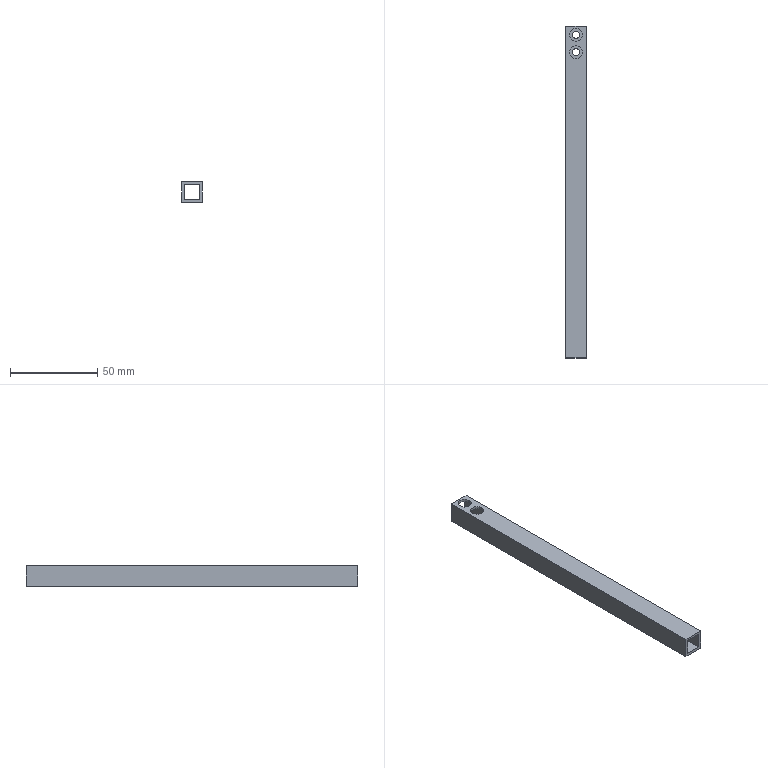Part | STEP file | B1-010 | 1 solid | 18 faces | box 12 x 190 x 12 mm | volume 11800 mm3 | plane 10 | cylinder 8 | commonest cylinder face diameters 4 x4 7.5 x4
STEP:
#1=CARTESIAN_POINT('',(0.,0.,0.));
#2=DIRECTION('',(0.,0.,1.));
#3=DIRECTION('',(1.,0.,0.));
#4=AXIS2_PLACEMENT_3D('',#1,#2,#3);
#5=CARTESIAN_POINT('',(3.75,80.,4.5));
#6=VERTEX_POINT('',#5);
#7=CARTESIAN_POINT('',(3.75,80.,6.));
#8=VERTEX_POINT('',#7);
#9=CARTESIAN_POINT('',(3.75,80.,-6.001));
#10=DIRECTION('',(0.,0.,1.));
#11=VECTOR('',#10,1.);
#12=LINE('',#9,#11);
#13=CARTESIAN_POINT('',(0.,80.,-6.001));
#14=DIRECTION('',(0.,0.,1.));
#15=DIRECTION('',(1.,0.,0.));
#16=AXIS2_PLACEMENT_3D('',#13,#14,#15);
#17=CYLINDRICAL_SURFACE('',#16,3.75);
#18=CARTESIAN_POINT('',(6.283,0.));
#19=DIRECTION('',(0.,1.));
#20=VECTOR('',#19,1.);
#21=LINE('',#18,#20);
#22=(GEOMETRIC_REPRESENTATION_CONTEXT(2)PARAMETRIC_REPRESENTATION_CONTEXT()REPRESENTATION_CONTEXT('',''));
#23=DEFINITIONAL_REPRESENTATION('',(#21),#22);
#24=PCURVE('',#17,#23);
#25=CARTESIAN_POINT('',(0.,80.,-6.001));
#26=DIRECTION('',(0.,0.,1.));
#27=DIRECTION('',(1.,0.,0.));
#28=AXIS2_PLACEMENT_3D('',#25,#26,#27);
#29=CYLINDRICAL_SURFACE('',#28,3.75);
#30=CARTESIAN_POINT('',(0.,0.));
#31=DIRECTION('',(0.,1.));
#32=VECTOR('',#31,1.);
#33=LINE('',#30,#32);
#34=(GEOMETRIC_REPRESENTATION_CONTEXT(2)PARAMETRIC_REPRESENTATION_CONTEXT()REPRESENTATION_CONTEXT('',''));
#35=DEFINITIONAL_REPRESENTATION('',(#33),#34);
#36=PCURVE('',#29,#35);
#37=SURFACE_CURVE('',#12,(#24,#36),.PCURVE_S1.);
#38=EDGE_CURVE('',#6,#8,#37,.T.);
#39=ORIENTED_EDGE('',*,*,#38,.T.);
#40=CARTESIAN_POINT('',(-3.75,80.,6.));
#41=VERTEX_POINT('',#40);
#42=CARTESIAN_POINT('',(0.,80.,6.));
#43=DIRECTION('',(0.,0.,1.));
#44=DIRECTION('',(1.,0.,0.));
#45=AXIS2_PLACEMENT_3D('',#42,#43,#44);
#46=CIRCLE('',#45,3.75);
#47=CARTESIAN_POINT('',(0.,12.001));
#48=DIRECTION('',(1.,0.));
#49=VECTOR('',#48,1.);
#50=LINE('',#47,#49);
#51=(GEOMETRIC_REPRESENTATION_CONTEXT(2)PARAMETRIC_REPRESENTATION_CONTEXT()REPRESENTATION_CONTEXT('',''));
#52=DEFINITIONAL_REPRESENTATION('',(#50),#51);
#53=PCURVE('',#17,#52);
#54=CARTESIAN_POINT('',(-6.,95.,6.));
#55=DIRECTION('',(0.,0.,-1.));
#56=DIRECTION('',(-1.,0.,0.));
#57=AXIS2_PLACEMENT_3D('',#54,#55,#56);
#58=PLANE('',#57);
#59=CARTESIAN_POINT('',(-9.75,-15.));
#60=CARTESIAN_POINT('',(-9.75,-8.505));
#61=CARTESIAN_POINT('',(-4.125,-11.752));
#62=CARTESIAN_POINT('',(1.5,-15.));
#63=CARTESIAN_POINT('',(-4.125,-18.248));
#64=CARTESIAN_POINT('',(-9.75,-21.495));
#65=CARTESIAN_POINT('',(-9.75,-15.));
#66=(BOUNDED_CURVE()B_SPLINE_CURVE(2,(#59,#60,#61,#62,#63,#64,#65),.UNSPECIFIED.,.T.,.F.)B_SPLINE_CURVE_WITH_KNOTS((1,2,2,2,2,1),(-2.094,0.,2.094,4.189,6.283,8.378),.UNSPECIFIED.)CURVE()GEOMETRIC_REPRESENTATION_ITEM()RATIONAL_B_SPLINE_CURVE((1.,0.5,1.,0.5,1.,0.5,1.))REPRESENTATION_ITEM(''));
#67=(GEOMETRIC_REPRESENTATION_CONTEXT(2)PARAMETRIC_REPRESENTATION_CONTEXT()REPRESENTATION_CONTEXT('',''));
#68=DEFINITIONAL_REPRESENTATION('',(#66),#67);
#69=PCURVE('',#58,#68);
#70=SURFACE_CURVE('',#46,(#53,#69),.PCURVE_S1.);
#71=EDGE_CURVE('',#41,#8,#70,.T.);
#72=ORIENTED_EDGE('',*,*,#71,.F.);
#73=CARTESIAN_POINT('',(-3.75,80.,4.5));
#74=VERTEX_POINT('',#73);
#75=CARTESIAN_POINT('',(-3.75,80.,-6.001));
#76=DIRECTION('',(0.,0.,1.));
#77=VECTOR('',#76,1.);
#78=LINE('',#75,#77);
#79=CARTESIAN_POINT('',(3.142,0.));
#80=DIRECTION('',(0.,1.));
#81=VECTOR('',#80,1.);
#82=LINE('',#79,#81);
#83=(GEOMETRIC_REPRESENTATION_CONTEXT(2)PARAMETRIC_REPRESENTATION_CONTEXT()REPRESENTATION_CONTEXT('',''));
#84=DEFINITIONAL_REPRESENTATION('',(#82),#83);
#85=PCURVE('',#17,#84);
#86=CARTESIAN_POINT('',(3.142,0.));
#87=DIRECTION('',(0.,1.));
#88=VECTOR('',#87,1.);
#89=LINE('',#86,#88);
#90=(GEOMETRIC_REPRESENTATION_CONTEXT(2)PARAMETRIC_REPRESENTATION_CONTEXT()REPRESENTATION_CONTEXT('',''));
#91=DEFINITIONAL_REPRESENTATION('',(#89),#90);
#92=PCURVE('',#29,#91);
#93=SURFACE_CURVE('',#78,(#85,#92),.PCURVE_S1.);
#94=EDGE_CURVE('',#74,#41,#93,.T.);
#95=ORIENTED_EDGE('',*,*,#94,.F.);
#96=CARTESIAN_POINT('',(0.,80.,4.5));
#97=DIRECTION('',(0.,0.,1.));
#98=DIRECTION('',(-1.,0.,0.));
#99=AXIS2_PLACEMENT_3D('',#96,#97,#98);
#100=CIRCLE('',#99,3.75);
#101=CARTESIAN_POINT('',(3.142,10.501));
#102=DIRECTION('',(1.,0.));
#103=VECTOR('',#102,1.);
#104=LINE('',#101,#103);
#105=(GEOMETRIC_REPRESENTATION_CONTEXT(2)PARAMETRIC_REPRESENTATION_CONTEXT()REPRESENTATION_CONTEXT('',''));
#106=DEFINITIONAL_REPRESENTATION('',(#104),#105);
#107=PCURVE('',#17,#106);
#108=CARTESIAN_POINT('',(-4.5,95.,4.5));
#109=DIRECTION('',(0.,0.,-1.));
#110=DIRECTION('',(-1.,0.,0.));
#111=AXIS2_PLACEMENT_3D('',#108,#109,#110);
#112=PLANE('',#111);
#113=CARTESIAN_POINT('',(-0.75,-15.));
#114=CARTESIAN_POINT('',(-0.75,-21.495));
#115=CARTESIAN_POINT('',(-6.375,-18.248));
#116=CARTESIAN_POINT('',(-12.,-15.));
#117=CARTESIAN_POINT('',(-6.375,-11.752));
#118=CARTESIAN_POINT('',(-0.75,-8.505));
#119=CARTESIAN_POINT('',(-0.75,-15.));
#120=(BOUNDED_CURVE()B_SPLINE_CURVE(2,(#113,#114,#115,#116,#117,#118,#119),.UNSPECIFIED.,.T.,.F.)B_SPLINE_CURVE_WITH_KNOTS((1,2,2,2,2,1),(-2.094,0.,2.094,4.189,6.283,8.378),.UNSPECIFIED.)CURVE()GEOMETRIC_REPRESENTATION_ITEM()RATIONAL_B_SPLINE_CURVE((1.,0.5,1.,0.5,1.,0.5,1.))REPRESENTATION_ITEM(''));
#121=(GEOMETRIC_REPRESENTATION_CONTEXT(2)PARAMETRIC_REPRESENTATION_CONTEXT()REPRESENTATION_CONTEXT('',''));
#122=DEFINITIONAL_REPRESENTATION('',(#120),#121);
#123=PCURVE('',#112,#122);
#124=SURFACE_CURVE('',#100,(#107,#123),.PCURVE_S1.);
#125=EDGE_CURVE('',#74,#6,#124,.T.);
#126=ORIENTED_EDGE('',*,*,#125,.T.);
#127=EDGE_LOOP('',(#39,#72,#95,#126));
#128=FACE_BOUND('',#127,.F.);
#129=ADVANCED_FACE('',(#128),#17,.F.);
#130=CARTESIAN_POINT('',(2.,80.,-6.));
#131=VERTEX_POINT('',#130);
#132=CARTESIAN_POINT('',(2.,80.,-4.5));
#133=VERTEX_POINT('',#132);
#134=CARTESIAN_POINT('',(2.,80.,-6.));
#135=DIRECTION('',(0.,0.,1.));
#136=VECTOR('',#135,1.);
#137=LINE('',#134,#136);
#138=CARTESIAN_POINT('',(0.,80.,-6.));
#139=DIRECTION('',(0.,0.,1.));
#140=DIRECTION('',(1.,0.,0.));
#141=AXIS2_PLACEMENT_3D('',#138,#139,#140);
#142=CYLINDRICAL_SURFACE('',#141,2.);
#143=CARTESIAN_POINT('',(6.283,0.));
#144=DIRECTION('',(0.,1.));
#145=VECTOR('',#144,1.);
#146=LINE('',#143,#145);
#147=(GEOMETRIC_REPRESENTATION_CONTEXT(2)PARAMETRIC_REPRESENTATION_CONTEXT()REPRESENTATION_CONTEXT('',''));
#148=DEFINITIONAL_REPRESENTATION('',(#146),#147);
#149=PCURVE('',#142,#148);
#150=CARTESIAN_POINT('',(0.,80.,-6.));
#151=DIRECTION('',(0.,0.,1.));
#152=DIRECTION('',(1.,0.,0.));
#153=AXIS2_PLACEMENT_3D('',#150,#151,#152);
#154=CYLINDRICAL_SURFACE('',#153,2.);
#155=CARTESIAN_POINT('',(0.,0.));
#156=DIRECTION('',(0.,1.));
#157=VECTOR('',#156,1.);
#158=LINE('',#155,#157);
#159=(GEOMETRIC_REPRESENTATION_CONTEXT(2)PARAMETRIC_REPRESENTATION_CONTEXT()REPRESENTATION_CONTEXT('',''));
#160=DEFINITIONAL_REPRESENTATION('',(#158),#159);
#161=PCURVE('',#154,#160);
#162=SURFACE_CURVE('',#137,(#149,#161),.PCURVE_S1.);
#163=EDGE_CURVE('',#131,#133,#162,.T.);
#164=ORIENTED_EDGE('',*,*,#163,.T.);
#165=CARTESIAN_POINT('',(-2.,80.,-4.5));
#166=VERTEX_POINT('',#165);
#167=CARTESIAN_POINT('',(0.,80.,-4.5));
#168=DIRECTION('',(0.,0.,1.));
#169=DIRECTION('',(1.,0.,0.));
#170=AXIS2_PLACEMENT_3D('',#167,#168,#169);
#171=CIRCLE('',#170,2.);
#172=CARTESIAN_POINT('',(0.,1.5));
#173=DIRECTION('',(1.,0.));
#174=VECTOR('',#173,1.);
#175=LINE('',#172,#174);
#176=(GEOMETRIC_REPRESENTATION_CONTEXT(2)PARAMETRIC_REPRESENTATION_CONTEXT()REPRESENTATION_CONTEXT('',''));
#177=DEFINITIONAL_REPRESENTATION('',(#175),#176);
#178=PCURVE('',#142,#177);
#179=CARTESIAN_POINT('',(-4.5,95.,-4.5));
#180=DIRECTION('',(0.,0.,1.));
#181=DIRECTION('',(1.,0.,0.));
#182=AXIS2_PLACEMENT_3D('',#179,#180,#181);
#183=PLANE('',#182);
#184=CARTESIAN_POINT('',(4.5,-15.));
#185=DIRECTION('',(1.,0.));
#186=AXIS2_PLACEMENT_2D('',#184,#185);
#187=CIRCLE('',#186,2.);
#188=(GEOMETRIC_REPRESENTATION_CONTEXT(2)PARAMETRIC_REPRESENTATION_CONTEXT()REPRESENTATION_CONTEXT('',''));
#189=DEFINITIONAL_REPRESENTATION('',(#187),#188);
#190=PCURVE('',#183,#189);
#191=SURFACE_CURVE('',#171,(#178,#190),.PCURVE_S1.);
#192=EDGE_CURVE('',#166,#133,#191,.T.);
#193=ORIENTED_EDGE('',*,*,#192,.F.);
#194=CARTESIAN_POINT('',(-2.,80.,-6.));
#195=VERTEX_POINT('',#194);
#196=CARTESIAN_POINT('',(-2.,80.,-6.));
#197=DIRECTION('',(0.,0.,1.));
#198=VECTOR('',#197,1.);
#199=LINE('',#196,#198);
#200=CARTESIAN_POINT('',(3.142,0.));
#201=DIRECTION('',(0.,1.));
#202=VECTOR('',#201,1.);
#203=LINE('',#200,#202);
#204=(GEOMETRIC_REPRESENTATION_CONTEXT(2)PARAMETRIC_REPRESENTATION_CONTEXT()REPRESENTATION_CONTEXT('',''));
#205=DEFINITIONAL_REPRESENTATION('',(#203),#204);
#206=PCURVE('',#142,#205);
#207=CARTESIAN_POINT('',(3.142,0.));
#208=DIRECTION('',(0.,1.));
#209=VECTOR('',#208,1.);
#210=LINE('',#207,#209);
#211=(GEOMETRIC_REPRESENTATION_CONTEXT(2)PARAMETRIC_REPRESENTATION_CONTEXT()REPRESENTATION_CONTEXT('',''));
#212=DEFINITIONAL_REPRESENTATION('',(#210),#211);
#213=PCURVE('',#154,#212);
#214=SURFACE_CURVE('',#199,(#206,#213),.PCURVE_S1.);
#215=EDGE_CURVE('',#195,#166,#214,.T.);
#216=ORIENTED_EDGE('',*,*,#215,.F.);
#217=CARTESIAN_POINT('',(0.,80.,-6.));
#218=DIRECTION('',(0.,0.,1.));
#219=DIRECTION('',(1.,0.,0.));
#220=AXIS2_PLACEMENT_3D('',#217,#218,#219);
#221=CIRCLE('',#220,2.);
#222=CARTESIAN_POINT('',(0.,0.));
#223=DIRECTION('',(1.,0.));
#224=VECTOR('',#223,1.);
#225=LINE('',#222,#224);
#226=(GEOMETRIC_REPRESENTATION_CONTEXT(2)PARAMETRIC_REPRESENTATION_CONTEXT()REPRESENTATION_CONTEXT('',''));
#227=DEFINITIONAL_REPRESENTATION('',(#225),#226);
#228=PCURVE('',#142,#227);
#229=CARTESIAN_POINT('',(-6.,95.,-6.));
#230=DIRECTION('',(0.,0.,1.));
#231=DIRECTION('',(1.,0.,0.));
#232=AXIS2_PLACEMENT_3D('',#229,#230,#231);
#233=PLANE('',#232);
#234=CARTESIAN_POINT('',(6.,-15.));
#235=DIRECTION('',(1.,0.));
#236=AXIS2_PLACEMENT_2D('',#234,#235);
#237=CIRCLE('',#236,2.);
#238=(GEOMETRIC_REPRESENTATION_CONTEXT(2)PARAMETRIC_REPRESENTATION_CONTEXT()REPRESENTATION_CONTEXT('',''));
#239=DEFINITIONAL_REPRESENTATION('',(#237),#238);
#240=PCURVE('',#233,#239);
#241=SURFACE_CURVE('',#221,(#228,#240),.PCURVE_S1.);
#242=EDGE_CURVE('',#195,#131,#241,.T.);
#243=ORIENTED_EDGE('',*,*,#242,.T.);
#244=EDGE_LOOP('',(#164,#193,#216,#243));
#245=FACE_BOUND('',#244,.F.);
#246=ADVANCED_FACE('',(#245),#142,.F.);
#247=CARTESIAN_POINT('',(3.75,90.,4.5));
#248=VERTEX_POINT('',#247);
#249=CARTESIAN_POINT('',(3.75,90.,6.));
#250=VERTEX_POINT('',#249);
#251=CARTESIAN_POINT('',(3.75,90.,-6.001));
#252=DIRECTION('',(0.,0.,1.));
#253=VECTOR('',#252,1.);
#254=LINE('',#251,#253);
#255=CARTESIAN_POINT('',(0.,90.,-6.001));
#256=DIRECTION('',(0.,0.,1.));
#257=DIRECTION('',(1.,0.,0.));
#258=AXIS2_PLACEMENT_3D('',#255,#256,#257);
#259=CYLINDRICAL_SURFACE('',#258,3.75);
#260=CARTESIAN_POINT('',(6.283,0.));
#261=DIRECTION('',(0.,1.));
#262=VECTOR('',#261,1.);
#263=LINE('',#260,#262);
#264=(GEOMETRIC_REPRESENTATION_CONTEXT(2)PARAMETRIC_REPRESENTATION_CONTEXT()REPRESENTATION_CONTEXT('',''));
#265=DEFINITIONAL_REPRESENTATION('',(#263),#264);
#266=PCURVE('',#259,#265);
#267=CARTESIAN_POINT('',(0.,90.,-6.001));
#268=DIRECTION('',(0.,0.,1.));
#269=DIRECTION('',(1.,0.,0.));
#270=AXIS2_PLACEMENT_3D('',#267,#268,#269);
#271=CYLINDRICAL_SURFACE('',#270,3.75);
#272=CARTESIAN_POINT('',(0.,0.));
#273=DIRECTION('',(0.,1.));
#274=VECTOR('',#273,1.);
#275=LINE('',#272,#274);
#276=(GEOMETRIC_REPRESENTATION_CONTEXT(2)PARAMETRIC_REPRESENTATION_CONTEXT()REPRESENTATION_CONTEXT('',''));
#277=DEFINITIONAL_REPRESENTATION('',(#275),#276);
#278=PCURVE('',#271,#277);
#279=SURFACE_CURVE('',#254,(#266,#278),.PCURVE_S1.);
#280=EDGE_CURVE('',#248,#250,#279,.T.);
#281=ORIENTED_EDGE('',*,*,#280,.T.);
#282=CARTESIAN_POINT('',(-3.75,90.,6.));
#283=VERTEX_POINT('',#282);
#284=CARTESIAN_POINT('',(0.,90.,6.));
#285=DIRECTION('',(0.,0.,1.));
#286=DIRECTION('',(1.,0.,0.));
#287=AXIS2_PLACEMENT_3D('',#284,#285,#286);
#288=CIRCLE('',#287,3.75);
#289=CARTESIAN_POINT('',(0.,12.001));
#290=DIRECTION('',(1.,0.));
#291=VECTOR('',#290,1.);
#292=LINE('',#289,#291);
#293=(GEOMETRIC_REPRESENTATION_CONTEXT(2)PARAMETRIC_REPRESENTATION_CONTEXT()REPRESENTATION_CONTEXT('',''));
#294=DEFINITIONAL_REPRESENTATION('',(#292),#293);
#295=PCURVE('',#259,#294);
#296=CARTESIAN_POINT('',(-9.75,-5.));
#297=CARTESIAN_POINT('',(-9.75,1.495));
#298=CARTESIAN_POINT('',(-4.125,-1.752));
#299=CARTESIAN_POINT('',(1.5,-5.));
#300=CARTESIAN_POINT('',(-4.125,-8.248));
#301=CARTESIAN_POINT('',(-9.75,-11.495));
#302=CARTESIAN_POINT('',(-9.75,-5.));
#303=(BOUNDED_CURVE()B_SPLINE_CURVE(2,(#296,#297,#298,#299,#300,#301,#302),.UNSPECIFIED.,.T.,.F.)B_SPLINE_CURVE_WITH_KNOTS((1,2,2,2,2,1),(-2.094,0.,2.094,4.189,6.283,8.378),.UNSPECIFIED.)CURVE()GEOMETRIC_REPRESENTATION_ITEM()RATIONAL_B_SPLINE_CURVE((1.,0.5,1.,0.5,1.,0.5,1.))REPRESENTATION_ITEM(''));
#304=(GEOMETRIC_REPRESENTATION_CONTEXT(2)PARAMETRIC_REPRESENTATION_CONTEXT()REPRESENTATION_CONTEXT('',''));
#305=DEFINITIONAL_REPRESENTATION('',(#303),#304);
#306=PCURVE('',#58,#305);
#307=SURFACE_CURVE('',#288,(#295,#306),.PCURVE_S1.);
#308=EDGE_CURVE('',#283,#250,#307,.T.);
#309=ORIENTED_EDGE('',*,*,#308,.F.);
#310=CARTESIAN_POINT('',(-3.75,90.,4.5));
#311=VERTEX_POINT('',#310);
#312=CARTESIAN_POINT('',(-3.75,90.,-6.001));
#313=DIRECTION('',(0.,0.,1.));
#314=VECTOR('',#313,1.);
#315=LINE('',#312,#314);
#316=CARTESIAN_POINT('',(3.142,0.));
#317=DIRECTION('',(0.,1.));
#318=VECTOR('',#317,1.);
#319=LINE('',#316,#318);
#320=(GEOMETRIC_REPRESENTATION_CONTEXT(2)PARAMETRIC_REPRESENTATION_CONTEXT()REPRESENTATION_CONTEXT('',''));
#321=DEFINITIONAL_REPRESENTATION('',(#319),#320);
#322=PCURVE('',#259,#321);
#323=CARTESIAN_POINT('',(3.142,0.));
#324=DIRECTION('',(0.,1.));
#325=VECTOR('',#324,1.);
#326=LINE('',#323,#325);
#327=(GEOMETRIC_REPRESENTATION_CONTEXT(2)PARAMETRIC_REPRESENTATION_CONTEXT()REPRESENTATION_CONTEXT('',''));
#328=DEFINITIONAL_REPRESENTATION('',(#326),#327);
#329=PCURVE('',#271,#328);
#330=SURFACE_CURVE('',#315,(#322,#329),.PCURVE_S1.);
#331=EDGE_CURVE('',#311,#283,#330,.T.);
#332=ORIENTED_EDGE('',*,*,#331,.F.);
#333=CARTESIAN_POINT('',(0.,90.,4.5));
#334=DIRECTION('',(0.,0.,1.));
#335=DIRECTION('',(-1.,0.,0.));
#336=AXIS2_PLACEMENT_3D('',#333,#334,#335);
#337=CIRCLE('',#336,3.75);
#338=CARTESIAN_POINT('',(3.142,10.501));
#339=DIRECTION('',(1.,0.));
#340=VECTOR('',#339,1.);
#341=LINE('',#338,#340);
#342=(GEOMETRIC_REPRESENTATION_CONTEXT(2)PARAMETRIC_REPRESENTATION_CONTEXT()REPRESENTATION_CONTEXT('',''));
#343=DEFINITIONAL_REPRESENTATION('',(#341),#342);
#344=PCURVE('',#259,#343);
#345=CARTESIAN_POINT('',(-0.75,-5.));
#346=CARTESIAN_POINT('',(-0.75,-11.495));
#347=CARTESIAN_POINT('',(-6.375,-8.248));
#348=CARTESIAN_POINT('',(-12.,-5.));
#349=CARTESIAN_POINT('',(-6.375,-1.752));
#350=CARTESIAN_POINT('',(-0.75,1.495));
#351=CARTESIAN_POINT('',(-0.75,-5.));
#352=(BOUNDED_CURVE()B_SPLINE_CURVE(2,(#345,#346,#347,#348,#349,#350,#351),.UNSPECIFIED.,.T.,.F.)B_SPLINE_CURVE_WITH_KNOTS((1,2,2,2,2,1),(-2.094,0.,2.094,4.189,6.283,8.378),.UNSPECIFIED.)CURVE()GEOMETRIC_REPRESENTATION_ITEM()RATIONAL_B_SPLINE_CURVE((1.,0.5,1.,0.5,1.,0.5,1.))REPRESENTATION_ITEM(''));
#353=(GEOMETRIC_REPRESENTATION_CONTEXT(2)PARAMETRIC_REPRESENTATION_CONTEXT()REPRESENTATION_CONTEXT('',''));
#354=DEFINITIONAL_REPRESENTATION('',(#352),#353);
#355=PCURVE('',#112,#354);
#356=SURFACE_CURVE('',#337,(#344,#355),.PCURVE_S1.);
#357=EDGE_CURVE('',#311,#248,#356,.T.);
#358=ORIENTED_EDGE('',*,*,#357,.T.);
#359=EDGE_LOOP('',(#281,#309,#332,#358));
#360=FACE_BOUND('',#359,.F.);
#361=ADVANCED_FACE('',(#360),#259,.F.);
#362=CARTESIAN_POINT('',(2.,90.,-6.));
#363=VERTEX_POINT('',#362);
#364=CARTESIAN_POINT('',(2.,90.,-4.5));
#365=VERTEX_POINT('',#364);
#366=CARTESIAN_POINT('',(2.,90.,-6.));
#367=DIRECTION('',(0.,0.,1.));
#368=VECTOR('',#367,1.);
#369=LINE('',#366,#368);
#370=CARTESIAN_POINT('',(0.,90.,-6.));
#371=DIRECTION('',(0.,0.,1.));
#372=DIRECTION('',(1.,0.,0.));
#373=AXIS2_PLACEMENT_3D('',#370,#371,#372);
#374=CYLINDRICAL_SURFACE('',#373,2.);
#375=CARTESIAN_POINT('',(6.283,0.));
#376=DIRECTION('',(0.,1.));
#377=VECTOR('',#376,1.);
#378=LINE('',#375,#377);
#379=(GEOMETRIC_REPRESENTATION_CONTEXT(2)PARAMETRIC_REPRESENTATION_CONTEXT()REPRESENTATION_CONTEXT('',''));
#380=DEFINITIONAL_REPRESENTATION('',(#378),#379);
#381=PCURVE('',#374,#380);
#382=CARTESIAN_POINT('',(0.,90.,-6.));
#383=DIRECTION('',(0.,0.,1.));
#384=DIRECTION('',(1.,0.,0.));
#385=AXIS2_PLACEMENT_3D('',#382,#383,#384);
#386=CYLINDRICAL_SURFACE('',#385,2.);
#387=CARTESIAN_POINT('',(0.,0.));
#388=DIRECTION('',(0.,1.));
#389=VECTOR('',#388,1.);
#390=LINE('',#387,#389);
#391=(GEOMETRIC_REPRESENTATION_CONTEXT(2)PARAMETRIC_REPRESENTATION_CONTEXT()REPRESENTATION_CONTEXT('',''));
#392=DEFINITIONAL_REPRESENTATION('',(#390),#391);
#393=PCURVE('',#386,#392);
#394=SURFACE_CURVE('',#369,(#381,#393),.PCURVE_S1.);
#395=EDGE_CURVE('',#363,#365,#394,.T.);
#396=ORIENTED_EDGE('',*,*,#395,.T.);
#397=CARTESIAN_POINT('',(-2.,90.,-4.5));
#398=VERTEX_POINT('',#397);
#399=CARTESIAN_POINT('',(0.,90.,-4.5));
#400=DIRECTION('',(0.,0.,1.));
#401=DIRECTION('',(1.,0.,0.));
#402=AXIS2_PLACEMENT_3D('',#399,#400,#401);
#403=CIRCLE('',#402,2.);
#404=CARTESIAN_POINT('',(0.,1.5));
#405=DIRECTION('',(1.,0.));
#406=VECTOR('',#405,1.);
#407=LINE('',#404,#406);
#408=(GEOMETRIC_REPRESENTATION_CONTEXT(2)PARAMETRIC_REPRESENTATION_CONTEXT()REPRESENTATION_CONTEXT('',''));
#409=DEFINITIONAL_REPRESENTATION('',(#407),#408);
#410=PCURVE('',#374,#409);
#411=CARTESIAN_POINT('',(4.5,-5.));
#412=DIRECTION('',(1.,0.));
#413=AXIS2_PLACEMENT_2D('',#411,#412);
#414=CIRCLE('',#413,2.);
#415=(GEOMETRIC_REPRESENTATION_CONTEXT(2)PARAMETRIC_REPRESENTATION_CONTEXT()REPRESENTATION_CONTEXT('',''));
#416=DEFINITIONAL_REPRESENTATION('',(#414),#415);
#417=PCURVE('',#183,#416);
#418=SURFACE_CURVE('',#403,(#410,#417),.PCURVE_S1.);
#419=EDGE_CURVE('',#398,#365,#418,.T.);
#420=ORIENTED_EDGE('',*,*,#419,.F.);
#421=CARTESIAN_POINT('',(-2.,90.,-6.));
#422=VERTEX_POINT('',#421);
#423=CARTESIAN_POINT('',(-2.,90.,-6.));
#424=DIRECTION('',(0.,0.,1.));
#425=VECTOR('',#424,1.);
#426=LINE('',#423,#425);
#427=CARTESIAN_POINT('',(3.142,0.));
#428=DIRECTION('',(0.,1.));
#429=VECTOR('',#428,1.);
#430=LINE('',#427,#429);
#431=(GEOMETRIC_REPRESENTATION_CONTEXT(2)PARAMETRIC_REPRESENTATION_CONTEXT()REPRESENTATION_CONTEXT('',''));
#432=DEFINITIONAL_REPRESENTATION('',(#430),#431);
#433=PCURVE('',#374,#432);
#434=CARTESIAN_POINT('',(3.142,0.));
#435=DIRECTION('',(0.,1.));
#436=VECTOR('',#435,1.);
#437=LINE('',#434,#436);
#438=(GEOMETRIC_REPRESENTATION_CONTEXT(2)PARAMETRIC_REPRESENTATION_CONTEXT()REPRESENTATION_CONTEXT('',''));
#439=DEFINITIONAL_REPRESENTATION('',(#437),#438);
#440=PCURVE('',#386,#439);
#441=SURFACE_CURVE('',#426,(#433,#440),.PCURVE_S1.);
#442=EDGE_CURVE('',#422,#398,#441,.T.);
#443=ORIENTED_EDGE('',*,*,#442,.F.);
#444=CARTESIAN_POINT('',(0.,90.,-6.));
#445=DIRECTION('',(0.,0.,1.));
#446=DIRECTION('',(1.,0.,0.));
#447=AXIS2_PLACEMENT_3D('',#444,#445,#446);
#448=CIRCLE('',#447,2.);
#449=CARTESIAN_POINT('',(0.,0.));
#450=DIRECTION('',(1.,0.));
#451=VECTOR('',#450,1.);
#452=LINE('',#449,#451);
#453=(GEOMETRIC_REPRESENTATION_CONTEXT(2)PARAMETRIC_REPRESENTATION_CONTEXT()REPRESENTATION_CONTEXT('',''));
#454=DEFINITIONAL_REPRESENTATION('',(#452),#453);
#455=PCURVE('',#374,#454);
#456=CARTESIAN_POINT('',(6.,-5.));
#457=DIRECTION('',(1.,0.));
#458=AXIS2_PLACEMENT_2D('',#456,#457);
#459=CIRCLE('',#458,2.);
#460=(GEOMETRIC_REPRESENTATION_CONTEXT(2)PARAMETRIC_REPRESENTATION_CONTEXT()REPRESENTATION_CONTEXT('',''));
#461=DEFINITIONAL_REPRESENTATION('',(#459),#460);
#462=PCURVE('',#233,#461);
#463=SURFACE_CURVE('',#448,(#455,#462),.PCURVE_S1.);
#464=EDGE_CURVE('',#422,#363,#463,.T.);
#465=ORIENTED_EDGE('',*,*,#464,.T.);
#466=EDGE_LOOP('',(#396,#420,#443,#465));
#467=FACE_BOUND('',#466,.F.);
#468=ADVANCED_FACE('',(#467),#374,.F.);
#469=CARTESIAN_POINT('',(6.,95.,6.));
#470=VERTEX_POINT('',#469);
#471=CARTESIAN_POINT('',(6.,95.,-6.));
#472=VERTEX_POINT('',#471);
#473=CARTESIAN_POINT('',(6.,95.,-6.));
#474=DIRECTION('',(0.,0.,-1.));
#475=VECTOR('',#474,1.);
#476=LINE('',#473,#475);
#477=CARTESIAN_POINT('',(0.,95.,0.));
#478=DIRECTION('',(0.,1.,0.));
#479=DIRECTION('',(0.,0.,1.));
#480=AXIS2_PLACEMENT_3D('',#477,#478,#479);
#481=PLANE('',#480);
#482=CARTESIAN_POINT('',(-6.,6.));
#483=DIRECTION('',(-1.,0.));
#484=VECTOR('',#483,1.);
#485=LINE('',#482,#484);
#486=(GEOMETRIC_REPRESENTATION_CONTEXT(2)PARAMETRIC_REPRESENTATION_CONTEXT()REPRESENTATION_CONTEXT('',''));
#487=DEFINITIONAL_REPRESENTATION('',(#485),#486);
#488=PCURVE('',#481,#487);
#489=CARTESIAN_POINT('',(6.,95.,-6.));
#490=DIRECTION('',(-1.,0.,0.));
#491=DIRECTION('',(0.,0.,1.));
#492=AXIS2_PLACEMENT_3D('',#489,#490,#491);
#493=PLANE('',#492);
#494=CARTESIAN_POINT('',(0.,0.));
#495=DIRECTION('',(-1.,0.));
#496=VECTOR('',#495,1.);
#497=LINE('',#494,#496);
#498=(GEOMETRIC_REPRESENTATION_CONTEXT(2)PARAMETRIC_REPRESENTATION_CONTEXT()REPRESENTATION_CONTEXT('',''));
#499=DEFINITIONAL_REPRESENTATION('',(#497),#498);
#500=PCURVE('',#493,#499);
#501=SURFACE_CURVE('',#476,(#488,#500),.PCURVE_S1.);
#502=EDGE_CURVE('',#470,#472,#501,.T.);
#503=ORIENTED_EDGE('',*,*,#502,.T.);
#504=CARTESIAN_POINT('',(-6.,95.,-6.));
#505=VERTEX_POINT('',#504);
#506=CARTESIAN_POINT('',(-6.,95.,-6.));
#507=DIRECTION('',(-1.,0.,0.));
#508=VECTOR('',#507,1.);
#509=LINE('',#506,#508);
#510=CARTESIAN_POINT('',(-6.,-6.));
#511=DIRECTION('',(0.,-1.));
#512=VECTOR('',#511,1.);
#513=LINE('',#510,#512);
#514=(GEOMETRIC_REPRESENTATION_CONTEXT(2)PARAMETRIC_REPRESENTATION_CONTEXT()REPRESENTATION_CONTEXT('',''));
#515=DEFINITIONAL_REPRESENTATION('',(#513),#514);
#516=PCURVE('',#481,#515);
#517=CARTESIAN_POINT('',(0.,0.));
#518=DIRECTION('',(-1.,0.));
#519=VECTOR('',#518,1.);
#520=LINE('',#517,#519);
#521=(GEOMETRIC_REPRESENTATION_CONTEXT(2)PARAMETRIC_REPRESENTATION_CONTEXT()REPRESENTATION_CONTEXT('',''));
#522=DEFINITIONAL_REPRESENTATION('',(#520),#521);
#523=PCURVE('',#233,#522);
#524=SURFACE_CURVE('',#509,(#516,#523),.PCURVE_S1.);
#525=EDGE_CURVE('',#472,#505,#524,.T.);
#526=ORIENTED_EDGE('',*,*,#525,.T.);
#527=CARTESIAN_POINT('',(-6.,95.,6.));
#528=VERTEX_POINT('',#527);
#529=CARTESIAN_POINT('',(-6.,95.,-6.));
#530=DIRECTION('',(0.,0.,1.));
#531=VECTOR('',#530,1.);
#532=LINE('',#529,#531);
#533=CARTESIAN_POINT('',(-6.,-6.));
#534=DIRECTION('',(1.,0.));
#535=VECTOR('',#534,1.);
#536=LINE('',#533,#535);
#537=(GEOMETRIC_REPRESENTATION_CONTEXT(2)PARAMETRIC_REPRESENTATION_CONTEXT()REPRESENTATION_CONTEXT('',''));
#538=DEFINITIONAL_REPRESENTATION('',(#536),#537);
#539=PCURVE('',#481,#538);
#540=CARTESIAN_POINT('',(-6.,95.,-6.));
#541=DIRECTION('',(1.,0.,0.));
#542=DIRECTION('',(0.,0.,-1.));
#543=AXIS2_PLACEMENT_3D('',#540,#541,#542);
#544=PLANE('',#543);
#545=CARTESIAN_POINT('',(0.,0.));
#546=DIRECTION('',(-1.,0.));
#547=VECTOR('',#546,1.);
#548=LINE('',#545,#547);
#549=(GEOMETRIC_REPRESENTATION_CONTEXT(2)PARAMETRIC_REPRESENTATION_CONTEXT()REPRESENTATION_CONTEXT('',''));
#550=DEFINITIONAL_REPRESENTATION('',(#548),#549);
#551=PCURVE('',#544,#550);
#552=SURFACE_CURVE('',#532,(#539,#551),.PCURVE_S1.);
#553=EDGE_CURVE('',#505,#528,#552,.T.);
#554=ORIENTED_EDGE('',*,*,#553,.T.);
#555=CARTESIAN_POINT('',(-6.,95.,6.));
#556=DIRECTION('',(1.,0.,0.));
#557=VECTOR('',#556,1.);
#558=LINE('',#555,#557);
#559=CARTESIAN_POINT('',(6.,-6.));
#560=DIRECTION('',(0.,1.));
#561=VECTOR('',#560,1.);
#562=LINE('',#559,#561);
#563=(GEOMETRIC_REPRESENTATION_CONTEXT(2)PARAMETRIC_REPRESENTATION_CONTEXT()REPRESENTATION_CONTEXT('',''));
#564=DEFINITIONAL_REPRESENTATION('',(#562),#563);
#565=PCURVE('',#481,#564);
#566=CARTESIAN_POINT('',(0.,0.));
#567=DIRECTION('',(-1.,0.));
#568=VECTOR('',#567,1.);
#569=LINE('',#566,#568);
#570=(GEOMETRIC_REPRESENTATION_CONTEXT(2)PARAMETRIC_REPRESENTATION_CONTEXT()REPRESENTATION_CONTEXT('',''));
#571=DEFINITIONAL_REPRESENTATION('',(#569),#570);
#572=PCURVE('',#58,#571);
#573=SURFACE_CURVE('',#558,(#565,#572),.PCURVE_S1.);
#574=EDGE_CURVE('',#528,#470,#573,.T.);
#575=ORIENTED_EDGE('',*,*,#574,.T.);
#576=EDGE_LOOP('',(#503,#526,#554,#575));
#577=FACE_BOUND('',#576,.T.);
#578=CARTESIAN_POINT('',(-4.5,95.,-4.5));
#579=VERTEX_POINT('',#578);
#580=CARTESIAN_POINT('',(-4.5,95.,4.5));
#581=VERTEX_POINT('',#580);
#582=CARTESIAN_POINT('',(-4.5,95.,-4.5));
#583=DIRECTION('',(0.,0.,1.));
#584=VECTOR('',#583,1.);
#585=LINE('',#582,#584);
#586=CARTESIAN_POINT('',(-4.5,-4.5));
#587=DIRECTION('',(1.,0.));
#588=VECTOR('',#587,1.);
#589=LINE('',#586,#588);
#590=(GEOMETRIC_REPRESENTATION_CONTEXT(2)PARAMETRIC_REPRESENTATION_CONTEXT()REPRESENTATION_CONTEXT('',''));
#591=DEFINITIONAL_REPRESENTATION('',(#589),#590);
#592=PCURVE('',#481,#591);
#593=CARTESIAN_POINT('',(-4.5,95.,-4.5));
#594=DIRECTION('',(1.,0.,0.));
#595=DIRECTION('',(0.,0.,-1.));
#596=AXIS2_PLACEMENT_3D('',#593,#594,#595);
#597=PLANE('',#596);
#598=CARTESIAN_POINT('',(0.,0.));
#599=DIRECTION('',(-1.,0.));
#600=VECTOR('',#599,1.);
#601=LINE('',#598,#600);
#602=(GEOMETRIC_REPRESENTATION_CONTEXT(2)PARAMETRIC_REPRESENTATION_CONTEXT()REPRESENTATION_CONTEXT('',''));
#603=DEFINITIONAL_REPRESENTATION('',(#601),#602);
#604=PCURVE('',#597,#603);
#605=SURFACE_CURVE('',#585,(#592,#604),.PCURVE_S1.);
#606=EDGE_CURVE('',#579,#581,#605,.T.);
#607=ORIENTED_EDGE('',*,*,#606,.F.);
#608=CARTESIAN_POINT('',(4.5,95.,-4.5));
#609=VERTEX_POINT('',#608);
#610=CARTESIAN_POINT('',(-4.5,95.,-4.5));
#611=DIRECTION('',(-1.,0.,0.));
#612=VECTOR('',#611,1.);
#613=LINE('',#610,#612);
#614=CARTESIAN_POINT('',(-4.5,-4.5));
#615=DIRECTION('',(0.,-1.));
#616=VECTOR('',#615,1.);
#617=LINE('',#614,#616);
#618=(GEOMETRIC_REPRESENTATION_CONTEXT(2)PARAMETRIC_REPRESENTATION_CONTEXT()REPRESENTATION_CONTEXT('',''));
#619=DEFINITIONAL_REPRESENTATION('',(#617),#618);
#620=PCURVE('',#481,#619);
#621=CARTESIAN_POINT('',(0.,0.));
#622=DIRECTION('',(-1.,0.));
#623=VECTOR('',#622,1.);
#624=LINE('',#621,#623);
#625=(GEOMETRIC_REPRESENTATION_CONTEXT(2)PARAMETRIC_REPRESENTATION_CONTEXT()REPRESENTATION_CONTEXT('',''));
#626=DEFINITIONAL_REPRESENTATION('',(#624),#625);
#627=PCURVE('',#183,#626);
#628=SURFACE_CURVE('',#613,(#620,#627),.PCURVE_S1.);
#629=EDGE_CURVE('',#609,#579,#628,.T.);
#630=ORIENTED_EDGE('',*,*,#629,.F.);
#631=CARTESIAN_POINT('',(4.5,95.,4.5));
#632=VERTEX_POINT('',#631);
#633=CARTESIAN_POINT('',(4.5,95.,-4.5));
#634=DIRECTION('',(0.,0.,-1.));
#635=VECTOR('',#634,1.);
#636=LINE('',#633,#635);
#637=CARTESIAN_POINT('',(-4.5,4.5));
#638=DIRECTION('',(-1.,0.));
#639=VECTOR('',#638,1.);
#640=LINE('',#637,#639);
#641=(GEOMETRIC_REPRESENTATION_CONTEXT(2)PARAMETRIC_REPRESENTATION_CONTEXT()REPRESENTATION_CONTEXT('',''));
#642=DEFINITIONAL_REPRESENTATION('',(#640),#641);
#643=PCURVE('',#481,#642);
#644=CARTESIAN_POINT('',(4.5,95.,-4.5));
#645=DIRECTION('',(-1.,0.,0.));
#646=DIRECTION('',(0.,0.,1.));
#647=AXIS2_PLACEMENT_3D('',#644,#645,#646);
#648=PLANE('',#647);
#649=CARTESIAN_POINT('',(0.,0.));
#650=DIRECTION('',(-1.,0.));
#651=VECTOR('',#650,1.);
#652=LINE('',#649,#651);
#653=(GEOMETRIC_REPRESENTATION_CONTEXT(2)PARAMETRIC_REPRESENTATION_CONTEXT()REPRESENTATION_CONTEXT('',''));
#654=DEFINITIONAL_REPRESENTATION('',(#652),#653);
#655=PCURVE('',#648,#654);
#656=SURFACE_CURVE('',#636,(#643,#655),.PCURVE_S1.);
#657=EDGE_CURVE('',#632,#609,#656,.T.);
#658=ORIENTED_EDGE('',*,*,#657,.F.);
#659=CARTESIAN_POINT('',(-4.5,95.,4.5));
#660=DIRECTION('',(1.,0.,0.));
#661=VECTOR('',#660,1.);
#662=LINE('',#659,#661);
#663=CARTESIAN_POINT('',(4.5,-4.5));
#664=DIRECTION('',(0.,1.));
#665=VECTOR('',#664,1.);
#666=LINE('',#663,#665);
#667=(GEOMETRIC_REPRESENTATION_CONTEXT(2)PARAMETRIC_REPRESENTATION_CONTEXT()REPRESENTATION_CONTEXT('',''));
#668=DEFINITIONAL_REPRESENTATION('',(#666),#667);
#669=PCURVE('',#481,#668);
#670=CARTESIAN_POINT('',(0.,0.));
#671=DIRECTION('',(-1.,0.));
#672=VECTOR('',#671,1.);
#673=LINE('',#670,#672);
#674=(GEOMETRIC_REPRESENTATION_CONTEXT(2)PARAMETRIC_REPRESENTATION_CONTEXT()REPRESENTATION_CONTEXT('',''));
#675=DEFINITIONAL_REPRESENTATION('',(#673),#674);
#676=PCURVE('',#112,#675);
#677=SURFACE_CURVE('',#662,(#669,#676),.PCURVE_S1.);
#678=EDGE_CURVE('',#581,#632,#677,.T.);
#679=ORIENTED_EDGE('',*,*,#678,.F.);
#680=EDGE_LOOP('',(#607,#630,#658,#679));
#681=FACE_BOUND('',#680,.T.);
#682=ADVANCED_FACE('',(#577,#681),#481,.T.);
#683=CARTESIAN_POINT('',(6.,-95.,6.));
#684=VERTEX_POINT('',#683);
#685=CARTESIAN_POINT('',(6.,-95.,-6.));
#686=VERTEX_POINT('',#685);
#687=CARTESIAN_POINT('',(6.,-95.,-6.));
#688=DIRECTION('',(0.,0.,-1.));
#689=VECTOR('',#688,1.);
#690=LINE('',#687,#689);
#691=CARTESIAN_POINT('',(0.,-95.,0.));
#692=DIRECTION('',(0.,1.,0.));
#693=DIRECTION('',(0.,0.,1.));
#694=AXIS2_PLACEMENT_3D('',#691,#692,#693);
#695=PLANE('',#694);
#696=CARTESIAN_POINT('',(-6.,6.));
#697=DIRECTION('',(-1.,0.));
#698=VECTOR('',#697,1.);
#699=LINE('',#696,#698);
#700=(GEOMETRIC_REPRESENTATION_CONTEXT(2)PARAMETRIC_REPRESENTATION_CONTEXT()REPRESENTATION_CONTEXT('',''));
#701=DEFINITIONAL_REPRESENTATION('',(#699),#700);
#702=PCURVE('',#695,#701);
#703=CARTESIAN_POINT('',(0.,-190.));
#704=DIRECTION('',(-1.,0.));
#705=VECTOR('',#704,1.);
#706=LINE('',#703,#705);
#707=(GEOMETRIC_REPRESENTATION_CONTEXT(2)PARAMETRIC_REPRESENTATION_CONTEXT()REPRESENTATION_CONTEXT('',''));
#708=DEFINITIONAL_REPRESENTATION('',(#706),#707);
#709=PCURVE('',#493,#708);
#710=SURFACE_CURVE('',#690,(#702,#709),.PCURVE_S1.);
#711=EDGE_CURVE('',#684,#686,#710,.T.);
#712=ORIENTED_EDGE('',*,*,#711,.F.);
#713=CARTESIAN_POINT('',(-6.,-95.,6.));
#714=VERTEX_POINT('',#713);
#715=CARTESIAN_POINT('',(-6.,-95.,6.));
#716=DIRECTION('',(1.,0.,0.));
#717=VECTOR('',#716,1.);
#718=LINE('',#715,#717);
#719=CARTESIAN_POINT('',(6.,-6.));
#720=DIRECTION('',(0.,1.));
#721=VECTOR('',#720,1.);
#722=LINE('',#719,#721);
#723=(GEOMETRIC_REPRESENTATION_CONTEXT(2)PARAMETRIC_REPRESENTATION_CONTEXT()REPRESENTATION_CONTEXT('',''));
#724=DEFINITIONAL_REPRESENTATION('',(#722),#723);
#725=PCURVE('',#695,#724);
#726=CARTESIAN_POINT('',(0.,-190.));
#727=DIRECTION('',(-1.,0.));
#728=VECTOR('',#727,1.);
#729=LINE('',#726,#728);
#730=(GEOMETRIC_REPRESENTATION_CONTEXT(2)PARAMETRIC_REPRESENTATION_CONTEXT()REPRESENTATION_CONTEXT('',''));
#731=DEFINITIONAL_REPRESENTATION('',(#729),#730);
#732=PCURVE('',#58,#731);
#733=SURFACE_CURVE('',#718,(#725,#732),.PCURVE_S1.);
#734=EDGE_CURVE('',#714,#684,#733,.T.);
#735=ORIENTED_EDGE('',*,*,#734,.F.);
#736=CARTESIAN_POINT('',(-6.,-95.,-6.));
#737=VERTEX_POINT('',#736);
#738=CARTESIAN_POINT('',(-6.,-95.,-6.));
#739=DIRECTION('',(0.,0.,1.));
#740=VECTOR('',#739,1.);
#741=LINE('',#738,#740);
#742=CARTESIAN_POINT('',(-6.,-6.));
#743=DIRECTION('',(1.,0.));
#744=VECTOR('',#743,1.);
#745=LINE('',#742,#744);
#746=(GEOMETRIC_REPRESENTATION_CONTEXT(2)PARAMETRIC_REPRESENTATION_CONTEXT()REPRESENTATION_CONTEXT('',''));
#747=DEFINITIONAL_REPRESENTATION('',(#745),#746);
#748=PCURVE('',#695,#747);
#749=CARTESIAN_POINT('',(0.,-190.));
#750=DIRECTION('',(-1.,0.));
#751=VECTOR('',#750,1.);
#752=LINE('',#749,#751);
#753=(GEOMETRIC_REPRESENTATION_CONTEXT(2)PARAMETRIC_REPRESENTATION_CONTEXT()REPRESENTATION_CONTEXT('',''));
#754=DEFINITIONAL_REPRESENTATION('',(#752),#753);
#755=PCURVE('',#544,#754);
#756=SURFACE_CURVE('',#741,(#748,#755),.PCURVE_S1.);
#757=EDGE_CURVE('',#737,#714,#756,.T.);
#758=ORIENTED_EDGE('',*,*,#757,.F.);
#759=CARTESIAN_POINT('',(-6.,-95.,-6.));
#760=DIRECTION('',(-1.,0.,0.));
#761=VECTOR('',#760,1.);
#762=LINE('',#759,#761);
#763=CARTESIAN_POINT('',(-6.,-6.));
#764=DIRECTION('',(0.,-1.));
#765=VECTOR('',#764,1.);
#766=LINE('',#763,#765);
#767=(GEOMETRIC_REPRESENTATION_CONTEXT(2)PARAMETRIC_REPRESENTATION_CONTEXT()REPRESENTATION_CONTEXT('',''));
#768=DEFINITIONAL_REPRESENTATION('',(#766),#767);
#769=PCURVE('',#695,#768);
#770=CARTESIAN_POINT('',(0.,-190.));
#771=DIRECTION('',(-1.,0.));
#772=VECTOR('',#771,1.);
#773=LINE('',#770,#772);
#774=(GEOMETRIC_REPRESENTATION_CONTEXT(2)PARAMETRIC_REPRESENTATION_CONTEXT()REPRESENTATION_CONTEXT('',''));
#775=DEFINITIONAL_REPRESENTATION('',(#773),#774);
#776=PCURVE('',#233,#775);
#777=SURFACE_CURVE('',#762,(#769,#776),.PCURVE_S1.);
#778=EDGE_CURVE('',#686,#737,#777,.T.);
#779=ORIENTED_EDGE('',*,*,#778,.F.);
#780=EDGE_LOOP('',(#712,#735,#758,#779));
#781=FACE_BOUND('',#780,.T.);
#782=CARTESIAN_POINT('',(4.5,-95.,-4.5));
#783=VERTEX_POINT('',#782);
#784=CARTESIAN_POINT('',(-4.5,-95.,-4.5));
#785=VERTEX_POINT('',#784);
#786=CARTESIAN_POINT('',(-4.5,-95.,-4.5));
#787=DIRECTION('',(-1.,0.,0.));
#788=VECTOR('',#787,1.);
#789=LINE('',#786,#788);
#790=CARTESIAN_POINT('',(-4.5,-4.5));
#791=DIRECTION('',(0.,-1.));
#792=VECTOR('',#791,1.);
#793=LINE('',#790,#792);
#794=(GEOMETRIC_REPRESENTATION_CONTEXT(2)PARAMETRIC_REPRESENTATION_CONTEXT()REPRESENTATION_CONTEXT('',''));
#795=DEFINITIONAL_REPRESENTATION('',(#793),#794);
#796=PCURVE('',#695,#795);
#797=CARTESIAN_POINT('',(0.,-190.));
#798=DIRECTION('',(-1.,0.));
#799=VECTOR('',#798,1.);
#800=LINE('',#797,#799);
#801=(GEOMETRIC_REPRESENTATION_CONTEXT(2)PARAMETRIC_REPRESENTATION_CONTEXT()REPRESENTATION_CONTEXT('',''));
#802=DEFINITIONAL_REPRESENTATION('',(#800),#801);
#803=PCURVE('',#183,#802);
#804=SURFACE_CURVE('',#789,(#796,#803),.PCURVE_S1.);
#805=EDGE_CURVE('',#783,#785,#804,.T.);
#806=ORIENTED_EDGE('',*,*,#805,.T.);
#807=CARTESIAN_POINT('',(-4.5,-95.,4.5));
#808=VERTEX_POINT('',#807);
#809=CARTESIAN_POINT('',(-4.5,-95.,-4.5));
#810=DIRECTION('',(0.,0.,1.));
#811=VECTOR('',#810,1.);
#812=LINE('',#809,#811);
#813=CARTESIAN_POINT('',(-4.5,-4.5));
#814=DIRECTION('',(1.,0.));
#815=VECTOR('',#814,1.);
#816=LINE('',#813,#815);
#817=(GEOMETRIC_REPRESENTATION_CONTEXT(2)PARAMETRIC_REPRESENTATION_CONTEXT()REPRESENTATION_CONTEXT('',''));
#818=DEFINITIONAL_REPRESENTATION('',(#816),#817);
#819=PCURVE('',#695,#818);
#820=CARTESIAN_POINT('',(0.,-190.));
#821=DIRECTION('',(-1.,0.));
#822=VECTOR('',#821,1.);
#823=LINE('',#820,#822);
#824=(GEOMETRIC_REPRESENTATION_CONTEXT(2)PARAMETRIC_REPRESENTATION_CONTEXT()REPRESENTATION_CONTEXT('',''));
#825=DEFINITIONAL_REPRESENTATION('',(#823),#824);
#826=PCURVE('',#597,#825);
#827=SURFACE_CURVE('',#812,(#819,#826),.PCURVE_S1.);
#828=EDGE_CURVE('',#785,#808,#827,.T.);
#829=ORIENTED_EDGE('',*,*,#828,.T.);
#830=CARTESIAN_POINT('',(4.5,-95.,4.5));
#831=VERTEX_POINT('',#830);
#832=CARTESIAN_POINT('',(-4.5,-95.,4.5));
#833=DIRECTION('',(1.,0.,0.));
#834=VECTOR('',#833,1.);
#835=LINE('',#832,#834);
#836=CARTESIAN_POINT('',(4.5,-4.5));
#837=DIRECTION('',(0.,1.));
#838=VECTOR('',#837,1.);
#839=LINE('',#836,#838);
#840=(GEOMETRIC_REPRESENTATION_CONTEXT(2)PARAMETRIC_REPRESENTATION_CONTEXT()REPRESENTATION_CONTEXT('',''));
#841=DEFINITIONAL_REPRESENTATION('',(#839),#840);
#842=PCURVE('',#695,#841);
#843=CARTESIAN_POINT('',(0.,-190.));
#844=DIRECTION('',(-1.,0.));
#845=VECTOR('',#844,1.);
#846=LINE('',#843,#845);
#847=(GEOMETRIC_REPRESENTATION_CONTEXT(2)PARAMETRIC_REPRESENTATION_CONTEXT()REPRESENTATION_CONTEXT('',''));
#848=DEFINITIONAL_REPRESENTATION('',(#846),#847);
#849=PCURVE('',#112,#848);
#850=SURFACE_CURVE('',#835,(#842,#849),.PCURVE_S1.);
#851=EDGE_CURVE('',#808,#831,#850,.T.);
#852=ORIENTED_EDGE('',*,*,#851,.T.);
#853=CARTESIAN_POINT('',(4.5,-95.,-4.5));
#854=DIRECTION('',(0.,0.,-1.));
#855=VECTOR('',#854,1.);
#856=LINE('',#853,#855);
#857=CARTESIAN_POINT('',(-4.5,4.5));
#858=DIRECTION('',(-1.,0.));
#859=VECTOR('',#858,1.);
#860=LINE('',#857,#859);
#861=(GEOMETRIC_REPRESENTATION_CONTEXT(2)PARAMETRIC_REPRESENTATION_CONTEXT()REPRESENTATION_CONTEXT('',''));
#862=DEFINITIONAL_REPRESENTATION('',(#860),#861);
#863=PCURVE('',#695,#862);
#864=CARTESIAN_POINT('',(0.,-190.));
#865=DIRECTION('',(-1.,0.));
#866=VECTOR('',#865,1.);
#867=LINE('',#864,#866);
#868=(GEOMETRIC_REPRESENTATION_CONTEXT(2)PARAMETRIC_REPRESENTATION_CONTEXT()REPRESENTATION_CONTEXT('',''));
#869=DEFINITIONAL_REPRESENTATION('',(#867),#868);
#870=PCURVE('',#648,#869);
#871=SURFACE_CURVE('',#856,(#863,#870),.PCURVE_S1.);
#872=EDGE_CURVE('',#831,#783,#871,.T.);
#873=ORIENTED_EDGE('',*,*,#872,.T.);
#874=EDGE_LOOP('',(#806,#829,#852,#873));
#875=FACE_BOUND('',#874,.T.);
#876=ADVANCED_FACE('',(#781,#875),#695,.F.);
#877=ORIENTED_EDGE('',*,*,#711,.T.);
#878=CARTESIAN_POINT('',(6.,95.,-6.));
#879=DIRECTION('',(0.,-1.,0.));
#880=VECTOR('',#879,1.);
#881=LINE('',#878,#880);
#882=CARTESIAN_POINT('',(0.,0.));
#883=DIRECTION('',(0.,-1.));
#884=VECTOR('',#883,1.);
#885=LINE('',#882,#884);
#886=(GEOMETRIC_REPRESENTATION_CONTEXT(2)PARAMETRIC_REPRESENTATION_CONTEXT()REPRESENTATION_CONTEXT('',''));
#887=DEFINITIONAL_REPRESENTATION('',(#885),#886);
#888=PCURVE('',#493,#887);
#889=CARTESIAN_POINT('',(12.,0.));
#890=DIRECTION('',(0.,-1.));
#891=VECTOR('',#890,1.);
#892=LINE('',#889,#891);
#893=(GEOMETRIC_REPRESENTATION_CONTEXT(2)PARAMETRIC_REPRESENTATION_CONTEXT()REPRESENTATION_CONTEXT('',''));
#894=DEFINITIONAL_REPRESENTATION('',(#892),#893);
#895=PCURVE('',#233,#894);
#896=SURFACE_CURVE('',#881,(#888,#895),.PCURVE_S1.);
#897=EDGE_CURVE('',#472,#686,#896,.T.);
#898=ORIENTED_EDGE('',*,*,#897,.F.);
#899=ORIENTED_EDGE('',*,*,#502,.F.);
#900=CARTESIAN_POINT('',(6.,95.,6.));
#901=DIRECTION('',(0.,-1.,0.));
#902=VECTOR('',#901,1.);
#903=LINE('',#900,#902);
#904=CARTESIAN_POINT('',(12.,0.));
#905=DIRECTION('',(0.,-1.));
#906=VECTOR('',#905,1.);
#907=LINE('',#904,#906);
#908=(GEOMETRIC_REPRESENTATION_CONTEXT(2)PARAMETRIC_REPRESENTATION_CONTEXT()REPRESENTATION_CONTEXT('',''));
#909=DEFINITIONAL_REPRESENTATION('',(#907),#908);
#910=PCURVE('',#493,#909);
#911=CARTESIAN_POINT('',(-12.,0.));
#912=DIRECTION('',(0.,-1.));
#913=VECTOR('',#912,1.);
#914=LINE('',#911,#913);
#915=(GEOMETRIC_REPRESENTATION_CONTEXT(2)PARAMETRIC_REPRESENTATION_CONTEXT()REPRESENTATION_CONTEXT('',''));
#916=DEFINITIONAL_REPRESENTATION('',(#914),#915);
#917=PCURVE('',#58,#916);
#918=SURFACE_CURVE('',#903,(#910,#917),.PCURVE_S1.);
#919=EDGE_CURVE('',#470,#684,#918,.T.);
#920=ORIENTED_EDGE('',*,*,#919,.T.);
#921=EDGE_LOOP('',(#877,#898,#899,#920));
#922=FACE_BOUND('',#921,.T.);
#923=ADVANCED_FACE('',(#922),#493,.F.);
#924=CARTESIAN_POINT('',(0.,80.,-6.));
#925=DIRECTION('',(0.,0.,1.));
#926=DIRECTION('',(1.,0.,0.));
#927=AXIS2_PLACEMENT_3D('',#924,#925,#926);
#928=CIRCLE('',#927,2.);
#929=CARTESIAN_POINT('',(6.,-15.));
#930=DIRECTION('',(1.,0.));
#931=AXIS2_PLACEMENT_2D('',#929,#930);
#932=CIRCLE('',#931,2.);
#933=(GEOMETRIC_REPRESENTATION_CONTEXT(2)PARAMETRIC_REPRESENTATION_CONTEXT()REPRESENTATION_CONTEXT('',''));
#934=DEFINITIONAL_REPRESENTATION('',(#932),#933);
#935=PCURVE('',#233,#934);
#936=CARTESIAN_POINT('',(0.,0.));
#937=DIRECTION('',(1.,0.));
#938=VECTOR('',#937,1.);
#939=LINE('',#936,#938);
#940=(GEOMETRIC_REPRESENTATION_CONTEXT(2)PARAMETRIC_REPRESENTATION_CONTEXT()REPRESENTATION_CONTEXT('',''));
#941=DEFINITIONAL_REPRESENTATION('',(#939),#940);
#942=PCURVE('',#154,#941);
#943=SURFACE_CURVE('',#928,(#935,#942),.PCURVE_S1.);
#944=EDGE_CURVE('',#131,#195,#943,.T.);
#945=ORIENTED_EDGE('',*,*,#944,.T.);
#946=ORIENTED_EDGE('',*,*,#242,.T.);
#947=EDGE_LOOP('',(#945,#946));
#948=FACE_BOUND('',#947,.T.);
#949=CARTESIAN_POINT('',(0.,90.,-6.));
#950=DIRECTION('',(0.,0.,1.));
#951=DIRECTION('',(1.,0.,0.));
#952=AXIS2_PLACEMENT_3D('',#949,#950,#951);
#953=CIRCLE('',#952,2.);
#954=CARTESIAN_POINT('',(6.,-5.));
#955=DIRECTION('',(1.,0.));
#956=AXIS2_PLACEMENT_2D('',#954,#955);
#957=CIRCLE('',#956,2.);
#958=(GEOMETRIC_REPRESENTATION_CONTEXT(2)PARAMETRIC_REPRESENTATION_CONTEXT()REPRESENTATION_CONTEXT('',''));
#959=DEFINITIONAL_REPRESENTATION('',(#957),#958);
#960=PCURVE('',#233,#959);
#961=CARTESIAN_POINT('',(0.,0.));
#962=DIRECTION('',(1.,0.));
#963=VECTOR('',#962,1.);
#964=LINE('',#961,#963);
#965=(GEOMETRIC_REPRESENTATION_CONTEXT(2)PARAMETRIC_REPRESENTATION_CONTEXT()REPRESENTATION_CONTEXT('',''));
#966=DEFINITIONAL_REPRESENTATION('',(#964),#965);
#967=PCURVE('',#386,#966);
#968=SURFACE_CURVE('',#953,(#960,#967),.PCURVE_S1.);
#969=EDGE_CURVE('',#363,#422,#968,.T.);
#970=ORIENTED_EDGE('',*,*,#969,.T.);
#971=ORIENTED_EDGE('',*,*,#464,.T.);
#972=EDGE_LOOP('',(#970,#971));
#973=FACE_BOUND('',#972,.T.);
#974=ORIENTED_EDGE('',*,*,#778,.T.);
#975=CARTESIAN_POINT('',(-6.,95.,-6.));
#976=DIRECTION('',(0.,-1.,0.));
#977=VECTOR('',#976,1.);
#978=LINE('',#975,#977);
#979=CARTESIAN_POINT('',(0.,0.));
#980=DIRECTION('',(0.,-1.));
#981=VECTOR('',#980,1.);
#982=LINE('',#979,#981);
#983=(GEOMETRIC_REPRESENTATION_CONTEXT(2)PARAMETRIC_REPRESENTATION_CONTEXT()REPRESENTATION_CONTEXT('',''));
#984=DEFINITIONAL_REPRESENTATION('',(#982),#983);
#985=PCURVE('',#233,#984);
#986=CARTESIAN_POINT('',(0.,0.));
#987=DIRECTION('',(0.,-1.));
#988=VECTOR('',#987,1.);
#989=LINE('',#986,#988);
#990=(GEOMETRIC_REPRESENTATION_CONTEXT(2)PARAMETRIC_REPRESENTATION_CONTEXT()REPRESENTATION_CONTEXT('',''));
#991=DEFINITIONAL_REPRESENTATION('',(#989),#990);
#992=PCURVE('',#544,#991);
#993=SURFACE_CURVE('',#978,(#985,#992),.PCURVE_S1.);
#994=EDGE_CURVE('',#505,#737,#993,.T.);
#995=ORIENTED_EDGE('',*,*,#994,.F.);
#996=ORIENTED_EDGE('',*,*,#525,.F.);
#997=ORIENTED_EDGE('',*,*,#897,.T.);
#998=EDGE_LOOP('',(#974,#995,#996,#997));
#999=FACE_BOUND('',#998,.T.);
#1000=ADVANCED_FACE('',(#948,#973,#999),#233,.F.);
#1001=ORIENTED_EDGE('',*,*,#757,.T.);
#1002=CARTESIAN_POINT('',(-6.,95.,6.));
#1003=DIRECTION('',(0.,-1.,0.));
#1004=VECTOR('',#1003,1.);
#1005=LINE('',#1002,#1004);
#1006=CARTESIAN_POINT('',(-12.,0.));
#1007=DIRECTION('',(0.,-1.));
#1008=VECTOR('',#1007,1.);
#1009=LINE('',#1006,#1008);
#1010=(GEOMETRIC_REPRESENTATION_CONTEXT(2)PARAMETRIC_REPRESENTATION_CONTEXT()REPRESENTATION_CONTEXT('',''));
#1011=DEFINITIONAL_REPRESENTATION('',(#1009),#1010);
#1012=PCURVE('',#544,#1011);
#1013=CARTESIAN_POINT('',(0.,0.));
#1014=DIRECTION('',(0.,-1.));
#1015=VECTOR('',#1014,1.);
#1016=LINE('',#1013,#1015);
#1017=(GEOMETRIC_REPRESENTATION_CONTEXT(2)PARAMETRIC_REPRESENTATION_CONTEXT()REPRESENTATION_CONTEXT('',''));
#1018=DEFINITIONAL_REPRESENTATION('',(#1016),#1017);
#1019=PCURVE('',#58,#1018);
#1020=SURFACE_CURVE('',#1005,(#1012,#1019),.PCURVE_S1.);
#1021=EDGE_CURVE('',#528,#714,#1020,.T.);
#1022=ORIENTED_EDGE('',*,*,#1021,.F.);
#1023=ORIENTED_EDGE('',*,*,#553,.F.);
#1024=ORIENTED_EDGE('',*,*,#994,.T.);
#1025=EDGE_LOOP('',(#1001,#1022,#1023,#1024));
#1026=FACE_BOUND('',#1025,.T.);
#1027=ADVANCED_FACE('',(#1026),#544,.F.);
#1028=CARTESIAN_POINT('',(0.,80.,6.));
#1029=DIRECTION('',(0.,0.,1.));
#1030=DIRECTION('',(1.,0.,0.));
#1031=AXIS2_PLACEMENT_3D('',#1028,#1029,#1030);
#1032=CIRCLE('',#1031,3.75);
#1033=CARTESIAN_POINT('',(-9.75,-15.));
#1034=CARTESIAN_POINT('',(-9.75,-8.505));
#1035=CARTESIAN_POINT('',(-4.125,-11.752));
#1036=CARTESIAN_POINT('',(1.5,-15.));
#1037=CARTESIAN_POINT('',(-4.125,-18.248));
#1038=CARTESIAN_POINT('',(-9.75,-21.495));
#1039=CARTESIAN_POINT('',(-9.75,-15.));
#1040=(BOUNDED_CURVE()B_SPLINE_CURVE(2,(#1033,#1034,#1035,#1036,#1037,#1038,#1039),.UNSPECIFIED.,.T.,.F.)B_SPLINE_CURVE_WITH_KNOTS((1,2,2,2,2,1),(-2.094,0.,2.094,4.189,6.283,8.378),.UNSPECIFIED.)CURVE()GEOMETRIC_REPRESENTATION_ITEM()RATIONAL_B_SPLINE_CURVE((1.,0.5,1.,0.5,1.,0.5,1.))REPRESENTATION_ITEM(''));
#1041=(GEOMETRIC_REPRESENTATION_CONTEXT(2)PARAMETRIC_REPRESENTATION_CONTEXT()REPRESENTATION_CONTEXT('',''));
#1042=DEFINITIONAL_REPRESENTATION('',(#1040),#1041);
#1043=PCURVE('',#58,#1042);
#1044=CARTESIAN_POINT('',(0.,12.001));
#1045=DIRECTION('',(1.,0.));
#1046=VECTOR('',#1045,1.);
#1047=LINE('',#1044,#1046);
#1048=(GEOMETRIC_REPRESENTATION_CONTEXT(2)PARAMETRIC_REPRESENTATION_CONTEXT()REPRESENTATION_CONTEXT('',''));
#1049=DEFINITIONAL_REPRESENTATION('',(#1047),#1048);
#1050=PCURVE('',#29,#1049);
#1051=SURFACE_CURVE('',#1032,(#1043,#1050),.PCURVE_S1.);
#1052=EDGE_CURVE('',#8,#41,#1051,.T.);
#1053=ORIENTED_EDGE('',*,*,#1052,.F.);
#1054=ORIENTED_EDGE('',*,*,#71,.F.);
#1055=EDGE_LOOP('',(#1053,#1054));
#1056=FACE_BOUND('',#1055,.T.);
#1057=CARTESIAN_POINT('',(0.,90.,6.));
#1058=DIRECTION('',(0.,0.,1.));
#1059=DIRECTION('',(1.,0.,0.));
#1060=AXIS2_PLACEMENT_3D('',#1057,#1058,#1059);
#1061=CIRCLE('',#1060,3.75);
#1062=CARTESIAN_POINT('',(-9.75,-5.));
#1063=CARTESIAN_POINT('',(-9.75,1.495));
#1064=CARTESIAN_POINT('',(-4.125,-1.752));
#1065=CARTESIAN_POINT('',(1.5,-5.));
#1066=CARTESIAN_POINT('',(-4.125,-8.248));
#1067=CARTESIAN_POINT('',(-9.75,-11.495));
#1068=CARTESIAN_POINT('',(-9.75,-5.));
#1069=(BOUNDED_CURVE()B_SPLINE_CURVE(2,(#1062,#1063,#1064,#1065,#1066,#1067,#1068),.UNSPECIFIED.,.T.,.F.)B_SPLINE_CURVE_WITH_KNOTS((1,2,2,2,2,1),(-2.094,0.,2.094,4.189,6.283,8.378),.UNSPECIFIED.)CURVE()GEOMETRIC_REPRESENTATION_ITEM()RATIONAL_B_SPLINE_CURVE((1.,0.5,1.,0.5,1.,0.5,1.))REPRESENTATION_ITEM(''));
#1070=(GEOMETRIC_REPRESENTATION_CONTEXT(2)PARAMETRIC_REPRESENTATION_CONTEXT()REPRESENTATION_CONTEXT('',''));
#1071=DEFINITIONAL_REPRESENTATION('',(#1069),#1070);
#1072=PCURVE('',#58,#1071);
#1073=CARTESIAN_POINT('',(0.,12.001));
#1074=DIRECTION('',(1.,0.));
#1075=VECTOR('',#1074,1.);
#1076=LINE('',#1073,#1075);
#1077=(GEOMETRIC_REPRESENTATION_CONTEXT(2)PARAMETRIC_REPRESENTATION_CONTEXT()REPRESENTATION_CONTEXT('',''));
#1078=DEFINITIONAL_REPRESENTATION('',(#1076),#1077);
#1079=PCURVE('',#271,#1078);
#1080=SURFACE_CURVE('',#1061,(#1072,#1079),.PCURVE_S1.);
#1081=EDGE_CURVE('',#250,#283,#1080,.T.);
#1082=ORIENTED_EDGE('',*,*,#1081,.F.);
#1083=ORIENTED_EDGE('',*,*,#308,.F.);
#1084=EDGE_LOOP('',(#1082,#1083));
#1085=FACE_BOUND('',#1084,.T.);
#1086=ORIENTED_EDGE('',*,*,#734,.T.);
#1087=ORIENTED_EDGE('',*,*,#919,.F.);
#1088=ORIENTED_EDGE('',*,*,#574,.F.);
#1089=ORIENTED_EDGE('',*,*,#1021,.T.);
#1090=EDGE_LOOP('',(#1086,#1087,#1088,#1089));
#1091=FACE_BOUND('',#1090,.T.);
#1092=ADVANCED_FACE('',(#1056,#1085,#1091),#58,.F.);
#1093=CARTESIAN_POINT('',(0.,80.,-4.5));
#1094=DIRECTION('',(0.,0.,1.));
#1095=DIRECTION('',(1.,0.,0.));
#1096=AXIS2_PLACEMENT_3D('',#1093,#1094,#1095);
#1097=CIRCLE('',#1096,2.);
#1098=CARTESIAN_POINT('',(4.5,-15.));
#1099=DIRECTION('',(1.,0.));
#1100=AXIS2_PLACEMENT_2D('',#1098,#1099);
#1101=CIRCLE('',#1100,2.);
#1102=(GEOMETRIC_REPRESENTATION_CONTEXT(2)PARAMETRIC_REPRESENTATION_CONTEXT()REPRESENTATION_CONTEXT('',''));
#1103=DEFINITIONAL_REPRESENTATION('',(#1101),#1102);
#1104=PCURVE('',#183,#1103);
#1105=CARTESIAN_POINT('',(0.,1.5));
#1106=DIRECTION('',(1.,0.));
#1107=VECTOR('',#1106,1.);
#1108=LINE('',#1105,#1107);
#1109=(GEOMETRIC_REPRESENTATION_CONTEXT(2)PARAMETRIC_REPRESENTATION_CONTEXT()REPRESENTATION_CONTEXT('',''));
#1110=DEFINITIONAL_REPRESENTATION('',(#1108),#1109);
#1111=PCURVE('',#154,#1110);
#1112=SURFACE_CURVE('',#1097,(#1104,#1111),.PCURVE_S1.);
#1113=EDGE_CURVE('',#133,#166,#1112,.T.);
#1114=ORIENTED_EDGE('',*,*,#1113,.F.);
#1115=ORIENTED_EDGE('',*,*,#192,.F.);
#1116=EDGE_LOOP('',(#1114,#1115));
#1117=FACE_BOUND('',#1116,.T.);
#1118=CARTESIAN_POINT('',(0.,90.,-4.5));
#1119=DIRECTION('',(0.,0.,1.));
#1120=DIRECTION('',(1.,0.,0.));
#1121=AXIS2_PLACEMENT_3D('',#1118,#1119,#1120);
#1122=CIRCLE('',#1121,2.);
#1123=CARTESIAN_POINT('',(4.5,-5.));
#1124=DIRECTION('',(1.,0.));
#1125=AXIS2_PLACEMENT_2D('',#1123,#1124);
#1126=CIRCLE('',#1125,2.);
#1127=(GEOMETRIC_REPRESENTATION_CONTEXT(2)PARAMETRIC_REPRESENTATION_CONTEXT()REPRESENTATION_CONTEXT('',''));
#1128=DEFINITIONAL_REPRESENTATION('',(#1126),#1127);
#1129=PCURVE('',#183,#1128);
#1130=CARTESIAN_POINT('',(0.,1.5));
#1131=DIRECTION('',(1.,0.));
#1132=VECTOR('',#1131,1.);
#1133=LINE('',#1130,#1132);
#1134=(GEOMETRIC_REPRESENTATION_CONTEXT(2)PARAMETRIC_REPRESENTATION_CONTEXT()REPRESENTATION_CONTEXT('',''));
#1135=DEFINITIONAL_REPRESENTATION('',(#1133),#1134);
#1136=PCURVE('',#386,#1135);
#1137=SURFACE_CURVE('',#1122,(#1129,#1136),.PCURVE_S1.);
#1138=EDGE_CURVE('',#365,#398,#1137,.T.);
#1139=ORIENTED_EDGE('',*,*,#1138,.F.);
#1140=ORIENTED_EDGE('',*,*,#419,.F.);
#1141=EDGE_LOOP('',(#1139,#1140));
#1142=FACE_BOUND('',#1141,.T.);
#1143=ORIENTED_EDGE('',*,*,#805,.F.);
#1144=CARTESIAN_POINT('',(4.5,95.,-4.5));
#1145=DIRECTION('',(0.,-1.,0.));
#1146=VECTOR('',#1145,1.);
#1147=LINE('',#1144,#1146);
#1148=CARTESIAN_POINT('',(9.,0.));
#1149=DIRECTION('',(0.,-1.));
#1150=VECTOR('',#1149,1.);
#1151=LINE('',#1148,#1150);
#1152=(GEOMETRIC_REPRESENTATION_CONTEXT(2)PARAMETRIC_REPRESENTATION_CONTEXT()REPRESENTATION_CONTEXT('',''));
#1153=DEFINITIONAL_REPRESENTATION('',(#1151),#1152);
#1154=PCURVE('',#183,#1153);
#1155=CARTESIAN_POINT('',(0.,0.));
#1156=DIRECTION('',(0.,-1.));
#1157=VECTOR('',#1156,1.);
#1158=LINE('',#1155,#1157);
#1159=(GEOMETRIC_REPRESENTATION_CONTEXT(2)PARAMETRIC_REPRESENTATION_CONTEXT()REPRESENTATION_CONTEXT('',''));
#1160=DEFINITIONAL_REPRESENTATION('',(#1158),#1159);
#1161=PCURVE('',#648,#1160);
#1162=SURFACE_CURVE('',#1147,(#1154,#1161),.PCURVE_S1.);
#1163=EDGE_CURVE('',#609,#783,#1162,.T.);
#1164=ORIENTED_EDGE('',*,*,#1163,.F.);
#1165=ORIENTED_EDGE('',*,*,#629,.T.);
#1166=CARTESIAN_POINT('',(-4.5,95.,-4.5));
#1167=DIRECTION('',(0.,-1.,0.));
#1168=VECTOR('',#1167,1.);
#1169=LINE('',#1166,#1168);
#1170=CARTESIAN_POINT('',(0.,0.));
#1171=DIRECTION('',(0.,-1.));
#1172=VECTOR('',#1171,1.);
#1173=LINE('',#1170,#1172);
#1174=(GEOMETRIC_REPRESENTATION_CONTEXT(2)PARAMETRIC_REPRESENTATION_CONTEXT()REPRESENTATION_CONTEXT('',''));
#1175=DEFINITIONAL_REPRESENTATION('',(#1173),#1174);
#1176=PCURVE('',#183,#1175);
#1177=CARTESIAN_POINT('',(0.,0.));
#1178=DIRECTION('',(0.,-1.));
#1179=VECTOR('',#1178,1.);
#1180=LINE('',#1177,#1179);
#1181=(GEOMETRIC_REPRESENTATION_CONTEXT(2)PARAMETRIC_REPRESENTATION_CONTEXT()REPRESENTATION_CONTEXT('',''));
#1182=DEFINITIONAL_REPRESENTATION('',(#1180),#1181);
#1183=PCURVE('',#597,#1182);
#1184=SURFACE_CURVE('',#1169,(#1176,#1183),.PCURVE_S1.);
#1185=EDGE_CURVE('',#579,#785,#1184,.T.);
#1186=ORIENTED_EDGE('',*,*,#1185,.T.);
#1187=EDGE_LOOP('',(#1143,#1164,#1165,#1186));
#1188=FACE_BOUND('',#1187,.T.);
#1189=ADVANCED_FACE('',(#1117,#1142,#1188),#183,.T.);
#1190=ORIENTED_EDGE('',*,*,#828,.F.);
#1191=ORIENTED_EDGE('',*,*,#1185,.F.);
#1192=ORIENTED_EDGE('',*,*,#606,.T.);
#1193=CARTESIAN_POINT('',(-4.5,95.,4.5));
#1194=DIRECTION('',(0.,-1.,0.));
#1195=VECTOR('',#1194,1.);
#1196=LINE('',#1193,#1195);
#1197=CARTESIAN_POINT('',(-9.,0.));
#1198=DIRECTION('',(0.,-1.));
#1199=VECTOR('',#1198,1.);
#1200=LINE('',#1197,#1199);
#1201=(GEOMETRIC_REPRESENTATION_CONTEXT(2)PARAMETRIC_REPRESENTATION_CONTEXT()REPRESENTATION_CONTEXT('',''));
#1202=DEFINITIONAL_REPRESENTATION('',(#1200),#1201);
#1203=PCURVE('',#597,#1202);
#1204=CARTESIAN_POINT('',(0.,0.));
#1205=DIRECTION('',(0.,-1.));
#1206=VECTOR('',#1205,1.);
#1207=LINE('',#1204,#1206);
#1208=(GEOMETRIC_REPRESENTATION_CONTEXT(2)PARAMETRIC_REPRESENTATION_CONTEXT()REPRESENTATION_CONTEXT('',''));
#1209=DEFINITIONAL_REPRESENTATION('',(#1207),#1208);
#1210=PCURVE('',#112,#1209);
#1211=SURFACE_CURVE('',#1196,(#1203,#1210),.PCURVE_S1.);
#1212=EDGE_CURVE('',#581,#808,#1211,.T.);
#1213=ORIENTED_EDGE('',*,*,#1212,.T.);
#1214=EDGE_LOOP('',(#1190,#1191,#1192,#1213));
#1215=FACE_BOUND('',#1214,.T.);
#1216=ADVANCED_FACE('',(#1215),#597,.T.);
#1217=CARTESIAN_POINT('',(0.,80.,4.5));
#1218=DIRECTION('',(0.,0.,1.));
#1219=DIRECTION('',(-1.,0.,0.));
#1220=AXIS2_PLACEMENT_3D('',#1217,#1218,#1219);
#1221=CIRCLE('',#1220,3.75);
#1222=CARTESIAN_POINT('',(-0.75,-15.));
#1223=CARTESIAN_POINT('',(-0.75,-21.495));
#1224=CARTESIAN_POINT('',(-6.375,-18.248));
#1225=CARTESIAN_POINT('',(-12.,-15.));
#1226=CARTESIAN_POINT('',(-6.375,-11.752));
#1227=CARTESIAN_POINT('',(-0.75,-8.505));
#1228=CARTESIAN_POINT('',(-0.75,-15.));
#1229=(BOUNDED_CURVE()B_SPLINE_CURVE(2,(#1222,#1223,#1224,#1225,#1226,#1227,#1228),.UNSPECIFIED.,.T.,.F.)B_SPLINE_CURVE_WITH_KNOTS((1,2,2,2,2,1),(-2.094,0.,2.094,4.189,6.283,8.378),.UNSPECIFIED.)CURVE()GEOMETRIC_REPRESENTATION_ITEM()RATIONAL_B_SPLINE_CURVE((1.,0.5,1.,0.5,1.,0.5,1.))REPRESENTATION_ITEM(''));
#1230=(GEOMETRIC_REPRESENTATION_CONTEXT(2)PARAMETRIC_REPRESENTATION_CONTEXT()REPRESENTATION_CONTEXT('',''));
#1231=DEFINITIONAL_REPRESENTATION('',(#1229),#1230);
#1232=PCURVE('',#112,#1231);
#1233=CARTESIAN_POINT('',(-3.142,10.501));
#1234=DIRECTION('',(1.,0.));
#1235=VECTOR('',#1234,1.);
#1236=LINE('',#1233,#1235);
#1237=(GEOMETRIC_REPRESENTATION_CONTEXT(2)PARAMETRIC_REPRESENTATION_CONTEXT()REPRESENTATION_CONTEXT('',''));
#1238=DEFINITIONAL_REPRESENTATION('',(#1236),#1237);
#1239=PCURVE('',#29,#1238);
#1240=SURFACE_CURVE('',#1221,(#1232,#1239),.PCURVE_S1.);
#1241=EDGE_CURVE('',#6,#74,#1240,.T.);
#1242=ORIENTED_EDGE('',*,*,#1241,.T.);
#1243=ORIENTED_EDGE('',*,*,#125,.T.);
#1244=EDGE_LOOP('',(#1242,#1243));
#1245=FACE_BOUND('',#1244,.T.);
#1246=CARTESIAN_POINT('',(0.,90.,4.5));
#1247=DIRECTION('',(0.,0.,1.));
#1248=DIRECTION('',(-1.,0.,0.));
#1249=AXIS2_PLACEMENT_3D('',#1246,#1247,#1248);
#1250=CIRCLE('',#1249,3.75);
#1251=CARTESIAN_POINT('',(-0.75,-5.));
#1252=CARTESIAN_POINT('',(-0.75,-11.495));
#1253=CARTESIAN_POINT('',(-6.375,-8.248));
#1254=CARTESIAN_POINT('',(-12.,-5.));
#1255=CARTESIAN_POINT('',(-6.375,-1.752));
#1256=CARTESIAN_POINT('',(-0.75,1.495));
#1257=CARTESIAN_POINT('',(-0.75,-5.));
#1258=(BOUNDED_CURVE()B_SPLINE_CURVE(2,(#1251,#1252,#1253,#1254,#1255,#1256,#1257),.UNSPECIFIED.,.T.,.F.)B_SPLINE_CURVE_WITH_KNOTS((1,2,2,2,2,1),(-2.094,0.,2.094,4.189,6.283,8.378),.UNSPECIFIED.)CURVE()GEOMETRIC_REPRESENTATION_ITEM()RATIONAL_B_SPLINE_CURVE((1.,0.5,1.,0.5,1.,0.5,1.))REPRESENTATION_ITEM(''));
#1259=(GEOMETRIC_REPRESENTATION_CONTEXT(2)PARAMETRIC_REPRESENTATION_CONTEXT()REPRESENTATION_CONTEXT('',''));
#1260=DEFINITIONAL_REPRESENTATION('',(#1258),#1259);
#1261=PCURVE('',#112,#1260);
#1262=CARTESIAN_POINT('',(-3.142,10.501));
#1263=DIRECTION('',(1.,0.));
#1264=VECTOR('',#1263,1.);
#1265=LINE('',#1262,#1264);
#1266=(GEOMETRIC_REPRESENTATION_CONTEXT(2)PARAMETRIC_REPRESENTATION_CONTEXT()REPRESENTATION_CONTEXT('',''));
#1267=DEFINITIONAL_REPRESENTATION('',(#1265),#1266);
#1268=PCURVE('',#271,#1267);
#1269=SURFACE_CURVE('',#1250,(#1261,#1268),.PCURVE_S1.);
#1270=EDGE_CURVE('',#248,#311,#1269,.T.);
#1271=ORIENTED_EDGE('',*,*,#1270,.T.);
#1272=ORIENTED_EDGE('',*,*,#357,.T.);
#1273=EDGE_LOOP('',(#1271,#1272));
#1274=FACE_BOUND('',#1273,.T.);
#1275=ORIENTED_EDGE('',*,*,#851,.F.);
#1276=ORIENTED_EDGE('',*,*,#1212,.F.);
#1277=ORIENTED_EDGE('',*,*,#678,.T.);
#1278=CARTESIAN_POINT('',(4.5,95.,4.5));
#1279=DIRECTION('',(0.,-1.,0.));
#1280=VECTOR('',#1279,1.);
#1281=LINE('',#1278,#1280);
#1282=CARTESIAN_POINT('',(-9.,0.));
#1283=DIRECTION('',(0.,-1.));
#1284=VECTOR('',#1283,1.);
#1285=LINE('',#1282,#1284);
#1286=(GEOMETRIC_REPRESENTATION_CONTEXT(2)PARAMETRIC_REPRESENTATION_CONTEXT()REPRESENTATION_CONTEXT('',''));
#1287=DEFINITIONAL_REPRESENTATION('',(#1285),#1286);
#1288=PCURVE('',#112,#1287);
#1289=CARTESIAN_POINT('',(9.,0.));
#1290=DIRECTION('',(0.,-1.));
#1291=VECTOR('',#1290,1.);
#1292=LINE('',#1289,#1291);
#1293=(GEOMETRIC_REPRESENTATION_CONTEXT(2)PARAMETRIC_REPRESENTATION_CONTEXT()REPRESENTATION_CONTEXT('',''));
#1294=DEFINITIONAL_REPRESENTATION('',(#1292),#1293);
#1295=PCURVE('',#648,#1294);
#1296=SURFACE_CURVE('',#1281,(#1288,#1295),.PCURVE_S1.);
#1297=EDGE_CURVE('',#632,#831,#1296,.T.);
#1298=ORIENTED_EDGE('',*,*,#1297,.T.);
#1299=EDGE_LOOP('',(#1275,#1276,#1277,#1298));
#1300=FACE_BOUND('',#1299,.T.);
#1301=ADVANCED_FACE('',(#1245,#1274,#1300),#112,.T.);
#1302=ORIENTED_EDGE('',*,*,#872,.F.);
#1303=ORIENTED_EDGE('',*,*,#1297,.F.);
#1304=ORIENTED_EDGE('',*,*,#657,.T.);
#1305=ORIENTED_EDGE('',*,*,#1163,.T.);
#1306=EDGE_LOOP('',(#1302,#1303,#1304,#1305));
#1307=FACE_BOUND('',#1306,.T.);
#1308=ADVANCED_FACE('',(#1307),#648,.T.);
#1309=ORIENTED_EDGE('',*,*,#1138,.F.);
#1310=ORIENTED_EDGE('',*,*,#395,.F.);
#1311=ORIENTED_EDGE('',*,*,#969,.T.);
#1312=ORIENTED_EDGE('',*,*,#442,.T.);
#1313=EDGE_LOOP('',(#1309,#1310,#1311,#1312));
#1314=FACE_BOUND('',#1313,.F.);
#1315=ADVANCED_FACE('',(#1314),#386,.F.);
#1316=ORIENTED_EDGE('',*,*,#1081,.F.);
#1317=ORIENTED_EDGE('',*,*,#280,.F.);
#1318=ORIENTED_EDGE('',*,*,#1270,.T.);
#1319=ORIENTED_EDGE('',*,*,#331,.T.);
#1320=EDGE_LOOP('',(#1316,#1317,#1318,#1319));
#1321=FACE_BOUND('',#1320,.F.);
#1322=ADVANCED_FACE('',(#1321),#271,.F.);
#1323=ORIENTED_EDGE('',*,*,#1113,.F.);
#1324=ORIENTED_EDGE('',*,*,#163,.F.);
#1325=ORIENTED_EDGE('',*,*,#944,.T.);
#1326=ORIENTED_EDGE('',*,*,#215,.T.);
#1327=EDGE_LOOP('',(#1323,#1324,#1325,#1326));
#1328=FACE_BOUND('',#1327,.F.);
#1329=ADVANCED_FACE('',(#1328),#154,.F.);
#1330=ORIENTED_EDGE('',*,*,#1052,.F.);
#1331=ORIENTED_EDGE('',*,*,#38,.F.);
#1332=ORIENTED_EDGE('',*,*,#1241,.T.);
#1333=ORIENTED_EDGE('',*,*,#94,.T.);
#1334=EDGE_LOOP('',(#1330,#1331,#1332,#1333));
#1335=FACE_BOUND('',#1334,.F.);
#1336=ADVANCED_FACE('',(#1335),#29,.F.);
#1337=CLOSED_SHELL('',(#129,#246,#361,#468,#682,#876,#923,#1000,#1027,#1092,#1189,#1216,#1301,#1308,#1315,#1322,#1329,#1336));
#1338=MANIFOLD_SOLID_BREP('',#1337);
#1339=(LENGTH_UNIT()NAMED_UNIT(*)SI_UNIT(.MILLI.,.METRE.));
#1340=UNCERTAINTY_MEASURE_WITH_UNIT(LENGTH_MEASURE(0.0000001),#1339,'','');
#1341=(NAMED_UNIT(*)PLANE_ANGLE_UNIT()SI_UNIT($,.RADIAN.));
#1342=(NAMED_UNIT(*)SI_UNIT($,.STERADIAN.)SOLID_ANGLE_UNIT());
#1343=(GEOMETRIC_REPRESENTATION_CONTEXT(3)GLOBAL_UNCERTAINTY_ASSIGNED_CONTEXT((#1340))GLOBAL_UNIT_ASSIGNED_CONTEXT((#1339,#1341,#1342))REPRESENTATION_CONTEXT('',''));
#1344=ADVANCED_BREP_SHAPE_REPRESENTATION('',(#4,#1338),#1343);